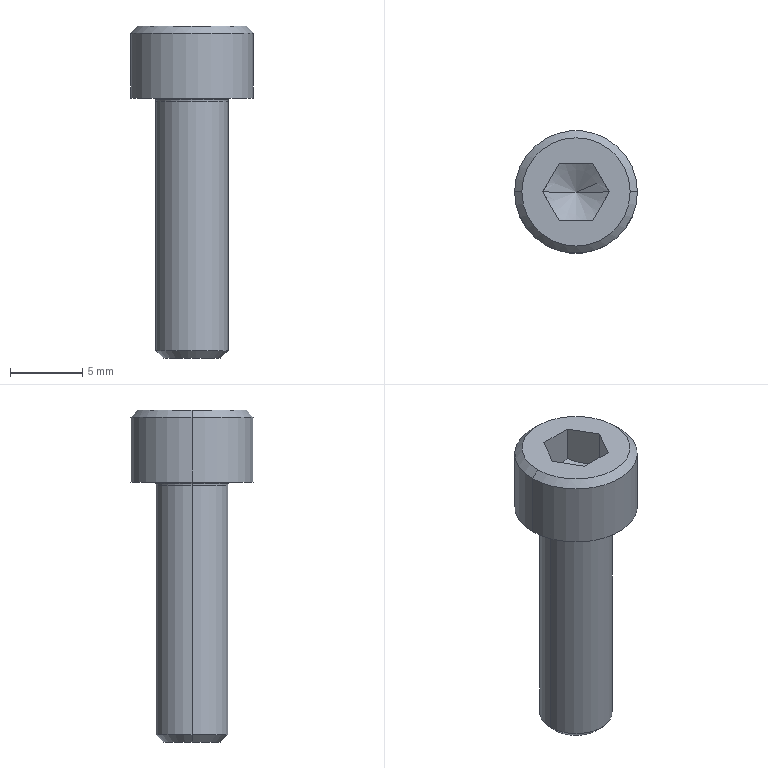Part | Creo | 1 solid | 23 faces | box 8.5 x 8.5 x 23 mm | volume 590.368 mm3 | plane 9 | cone 6 | cylinder 4 | torus 4 | commonest cylinder face diameters 5 x2 8.5 x2
STEP:
#1=CARTESIAN_POINT('',(-237.059,-351.009,-14.5));
#2=VERTEX_POINT('',#1);
#3=CARTESIAN_POINT('',(-238.214,-349.009,-14.5));
#4=VERTEX_POINT('',#3);
#5=CARTESIAN_POINT('',(-237.059,-351.009,-14.5));
#6=CARTESIAN_POINT('',(-237.113,-350.916,-14.531));
#7=CARTESIAN_POINT('',(-237.221,-350.729,-14.587));
#8=CARTESIAN_POINT('',(-237.386,-350.443,-14.648));
#9=CARTESIAN_POINT('',(-237.553,-350.153,-14.68));
#10=CARTESIAN_POINT('',(-237.72,-349.864,-14.68));
#11=CARTESIAN_POINT('',(-237.887,-349.575,-14.648));
#12=CARTESIAN_POINT('',(-238.053,-349.289,-14.587));
#13=CARTESIAN_POINT('',(-238.16,-349.102,-14.531));
#14=CARTESIAN_POINT('',(-238.214,-349.009,-14.5));
#15=B_SPLINE_CURVE_WITH_KNOTS('',3,(#5,#6,#7,#8,#9,#10,#11,#12,#13,#14),.UNSPECIFIED.,.F.,.F.,(4,1,1,1,1,1,1,4),(0.,0.1429,0.2857,0.4286,0.5714,0.7143,0.8571,1.),.UNSPECIFIED.);
#16=EDGE_CURVE('',#2,#4,#15,.T.);
#17=ORIENTED_EDGE('',*,*,#16,.F.);
#18=CARTESIAN_POINT('',(-239.368,-351.009,-15.833));
#19=VERTEX_POINT('',#18);
#20=CARTESIAN_POINT('',(-239.368,-351.009,-15.833));
#21=DIRECTION('',(0.866,0.,0.5));
#22=VECTOR('',#21,2.667);
#23=LINE('',#20,#22);
#24=EDGE_CURVE('',#19,#2,#23,.T.);
#25=ORIENTED_EDGE('',*,*,#24,.F.);
#26=CARTESIAN_POINT('',(-241.678,-351.009,-14.5));
#27=VERTEX_POINT('',#26);
#28=CARTESIAN_POINT('',(-239.368,-351.009,-15.833));
#29=DIRECTION('',(-0.866,0.,0.5));
#30=VECTOR('',#29,2.667);
#31=LINE('',#28,#30);
#32=EDGE_CURVE('',#19,#27,#31,.T.);
#33=ORIENTED_EDGE('',*,*,#32,.T.);
#34=CARTESIAN_POINT('',(-240.523,-349.009,-14.5));
#35=VERTEX_POINT('',#34);
#36=CARTESIAN_POINT('',(-240.523,-349.009,-14.5));
#37=CARTESIAN_POINT('',(-240.577,-349.102,-14.531));
#38=CARTESIAN_POINT('',(-240.685,-349.29,-14.587));
#39=CARTESIAN_POINT('',(-240.85,-349.576,-14.648));
#40=CARTESIAN_POINT('',(-241.017,-349.865,-14.68));
#41=CARTESIAN_POINT('',(-241.185,-350.155,-14.68));
#42=CARTESIAN_POINT('',(-241.351,-350.444,-14.648));
#43=CARTESIAN_POINT('',(-241.517,-350.73,-14.587));
#44=CARTESIAN_POINT('',(-241.624,-350.917,-14.531));
#45=CARTESIAN_POINT('',(-241.678,-351.009,-14.5));
#46=B_SPLINE_CURVE_WITH_KNOTS('',3,(#36,#37,#38,#39,#40,#41,#42,#43,#44,#45),.UNSPECIFIED.,.F.,.F.,(4,1,1,1,1,1,1,4),(0.,0.1429,0.2857,0.4286,0.5714,0.7143,0.8571,1.),.UNSPECIFIED.);
#47=EDGE_CURVE('',#35,#27,#46,.T.);
#48=ORIENTED_EDGE('',*,*,#47,.F.);
#49=CARTESIAN_POINT('',(-238.214,-349.009,-14.5));
#50=CARTESIAN_POINT('',(-238.276,-349.009,-14.518));
#51=CARTESIAN_POINT('',(-238.399,-349.009,-14.551));
#52=CARTESIAN_POINT('',(-238.576,-349.009,-14.592));
#53=CARTESIAN_POINT('',(-238.75,-349.009,-14.626));
#54=CARTESIAN_POINT('',(-238.924,-349.009,-14.652));
#55=CARTESIAN_POINT('',(-239.1,-349.009,-14.67));
#56=CARTESIAN_POINT('',(-239.279,-349.009,-14.679));
#57=CARTESIAN_POINT('',(-239.458,-349.009,-14.679));
#58=CARTESIAN_POINT('',(-239.636,-349.009,-14.67));
#59=CARTESIAN_POINT('',(-239.813,-349.009,-14.652));
#60=CARTESIAN_POINT('',(-239.987,-349.009,-14.626));
#61=CARTESIAN_POINT('',(-240.161,-349.009,-14.592));
#62=CARTESIAN_POINT('',(-240.338,-349.009,-14.551));
#63=CARTESIAN_POINT('',(-240.461,-349.009,-14.518));
#64=CARTESIAN_POINT('',(-240.523,-349.009,-14.5));
#65=B_SPLINE_CURVE_WITH_KNOTS('',3,(#49,#50,#51,#52,#53,#54,#55,#56,#57,#58,#59,#60,#61,#62,#63,#64),.UNSPECIFIED.,.F.,.F.,(4,1,1,1,1,1,1,1,1,1,1,1,1,4),(0.,0.07692,0.1538,0.2308,0.3077,0.3846,0.4615,0.5385,0.6154,0.6923,0.7692,0.8462,0.9231,1.),.UNSPECIFIED.);
#66=EDGE_CURVE('',#4,#35,#65,.T.);
#67=ORIENTED_EDGE('',*,*,#66,.F.);
#68=EDGE_LOOP('',(#17,#25,#33,#48,#67));
#69=FACE_OUTER_BOUND('',#68,.F.);
#70=CARTESIAN_POINT('',(-239.368,-351.009,-15.153));
#71=DIRECTION('',(0.,0.,1.));
#72=DIRECTION('',(1.,0.,0.));
#73=AXIS2_PLACEMENT_3D('',#70,#71,#72);
#74=CONICAL_SURFACE('',#73,1.178,60.);
#75=ADVANCED_FACE('',(#69),#74,.F.);
#76=CARTESIAN_POINT('',(-238.214,-349.009,-12.));
#77=VERTEX_POINT('',#76);
#78=CARTESIAN_POINT('',(-237.059,-351.009,-12.));
#79=VERTEX_POINT('',#78);
#80=CARTESIAN_POINT('',(-238.214,-349.009,-12.));
#81=DIRECTION('',(0.5,-0.866,0.));
#82=VECTOR('',#81,2.309);
#83=LINE('',#80,#82);
#84=EDGE_CURVE('',#77,#79,#83,.T.);
#85=ORIENTED_EDGE('',*,*,#84,.T.);
#86=CARTESIAN_POINT('',(-237.059,-351.009,-12.));
#87=DIRECTION('',(0.,0.,-1.));
#88=VECTOR('',#87,2.5);
#89=LINE('',#86,#88);
#90=EDGE_CURVE('',#79,#2,#89,.T.);
#91=ORIENTED_EDGE('',*,*,#90,.T.);
#92=ORIENTED_EDGE('',*,*,#16,.T.);
#93=CARTESIAN_POINT('',(-238.214,-349.009,-12.));
#94=DIRECTION('',(0.,0.,-1.));
#95=VECTOR('',#94,2.5);
#96=LINE('',#93,#95);
#97=EDGE_CURVE('',#77,#4,#96,.T.);
#98=ORIENTED_EDGE('',*,*,#97,.F.);
#99=EDGE_LOOP('',(#85,#91,#92,#98));
#100=FACE_OUTER_BOUND('',#99,.F.);
#101=CARTESIAN_POINT('',(-238.214,-349.009,-14.5));
#102=DIRECTION('',(-0.866,-0.5,0.));
#103=DIRECTION('',(0.5,-0.866,0.));
#104=AXIS2_PLACEMENT_3D('',#101,#102,#103);
#105=PLANE('',#104);
#106=ADVANCED_FACE('',(#100),#105,.T.);
#107=CARTESIAN_POINT('',(-235.618,-351.009,-12.));
#108=VERTEX_POINT('',#107);
#109=CARTESIAN_POINT('',(-243.118,-351.009,-12.));
#110=VERTEX_POINT('',#109);
#111=CARTESIAN_POINT('',(-239.368,-351.009,-12.));
#112=DIRECTION('',(0.,0.,1.));
#113=DIRECTION('',(1.,0.,0.));
#114=AXIS2_PLACEMENT_3D('',#111,#112,#113);
#115=CIRCLE('',#114,3.75);
#116=EDGE_CURVE('',#108,#110,#115,.T.);
#117=ORIENTED_EDGE('',*,*,#116,.F.);
#118=CARTESIAN_POINT('',(-239.368,-351.009,-12.));
#119=DIRECTION('',(0.,0.,1.));
#120=DIRECTION('',(-1.,0.,0.));
#121=AXIS2_PLACEMENT_3D('',#118,#119,#120);
#122=CIRCLE('',#121,3.75);
#123=EDGE_CURVE('',#110,#108,#122,.T.);
#124=ORIENTED_EDGE('',*,*,#123,.F.);
#125=EDGE_LOOP('',(#117,#124));
#126=FACE_OUTER_BOUND('',#125,.F.);
#127=CARTESIAN_POINT('',(-238.214,-353.009,-12.));
#128=VERTEX_POINT('',#127);
#129=CARTESIAN_POINT('',(-237.059,-351.009,-12.));
#130=DIRECTION('',(-0.5,-0.866,0.));
#131=VECTOR('',#130,2.309);
#132=LINE('',#129,#131);
#133=EDGE_CURVE('',#79,#128,#132,.T.);
#134=ORIENTED_EDGE('',*,*,#133,.F.);
#135=ORIENTED_EDGE('',*,*,#84,.F.);
#136=CARTESIAN_POINT('',(-240.523,-349.009,-12.));
#137=VERTEX_POINT('',#136);
#138=CARTESIAN_POINT('',(-238.214,-349.009,-12.));
#139=DIRECTION('',(-1.,0.,0.));
#140=VECTOR('',#139,2.309);
#141=LINE('',#138,#140);
#142=EDGE_CURVE('',#77,#137,#141,.T.);
#143=ORIENTED_EDGE('',*,*,#142,.T.);
#144=CARTESIAN_POINT('',(-241.678,-351.009,-12.));
#145=VERTEX_POINT('',#144);
#146=CARTESIAN_POINT('',(-241.678,-351.009,-12.));
#147=DIRECTION('',(0.5,0.866,0.));
#148=VECTOR('',#147,2.309);
#149=LINE('',#146,#148);
#150=EDGE_CURVE('',#145,#137,#149,.T.);
#151=ORIENTED_EDGE('',*,*,#150,.F.);
#152=CARTESIAN_POINT('',(-240.523,-353.009,-12.));
#153=VERTEX_POINT('',#152);
#154=CARTESIAN_POINT('',(-240.523,-353.009,-12.));
#155=DIRECTION('',(-0.5,0.866,0.));
#156=VECTOR('',#155,2.309);
#157=LINE('',#154,#156);
#158=EDGE_CURVE('',#153,#145,#157,.T.);
#159=ORIENTED_EDGE('',*,*,#158,.F.);
#160=CARTESIAN_POINT('',(-240.523,-353.009,-12.));
#161=DIRECTION('',(1.,0.,0.));
#162=VECTOR('',#161,2.309);
#163=LINE('',#160,#162);
#164=EDGE_CURVE('',#153,#128,#163,.T.);
#165=ORIENTED_EDGE('',*,*,#164,.T.);
#166=EDGE_LOOP('',(#134,#135,#143,#151,#159,#165));
#167=FACE_BOUND('',#166,.F.);
#168=CARTESIAN_POINT('',(-239.368,-351.009,-12.));
#169=DIRECTION('',(0.,0.,1.));
#170=DIRECTION('',(1.,0.,0.));
#171=AXIS2_PLACEMENT_3D('',#168,#169,#170);
#172=PLANE('',#171);
#173=ADVANCED_FACE('',(#126,#167),#172,.T.);
#174=CARTESIAN_POINT('',(-235.118,-351.009,-12.5));
#175=VERTEX_POINT('',#174);
#176=CARTESIAN_POINT('',(-243.618,-351.009,-12.5));
#177=VERTEX_POINT('',#176);
#178=CARTESIAN_POINT('',(-239.368,-351.009,-12.5));
#179=DIRECTION('',(0.,0.,1.));
#180=DIRECTION('',(1.,0.,0.));
#181=AXIS2_PLACEMENT_3D('',#178,#179,#180);
#182=CIRCLE('',#181,4.25);
#183=EDGE_CURVE('',#175,#177,#182,.T.);
#184=ORIENTED_EDGE('',*,*,#183,.F.);
#185=CARTESIAN_POINT('',(-235.618,-351.009,-12.));
#186=DIRECTION('',(0.7071,0.,-0.7071));
#187=VECTOR('',#186,0.7071);
#188=LINE('',#185,#187);
#189=EDGE_CURVE('',#108,#175,#188,.T.);
#190=ORIENTED_EDGE('',*,*,#189,.F.);
#191=ORIENTED_EDGE('',*,*,#116,.T.);
#192=CARTESIAN_POINT('',(-243.118,-351.009,-12.));
#193=DIRECTION('',(-0.7071,0.,-0.7071));
#194=VECTOR('',#193,0.7071);
#195=LINE('',#192,#194);
#196=EDGE_CURVE('',#110,#177,#195,.T.);
#197=ORIENTED_EDGE('',*,*,#196,.T.);
#198=EDGE_LOOP('',(#184,#190,#191,#197));
#199=FACE_OUTER_BOUND('',#198,.F.);
#200=CARTESIAN_POINT('',(-239.368,-351.009,-12.25));
#201=DIRECTION('',(0.,0.,-1.));
#202=DIRECTION('',(-1.,0.,0.));
#203=AXIS2_PLACEMENT_3D('',#200,#201,#202);
#204=CONICAL_SURFACE('',#203,4.,45.);
#205=ADVANCED_FACE('',(#199),#204,.T.);
#206=ORIENTED_EDGE('',*,*,#183,.T.);
#207=CARTESIAN_POINT('',(-243.618,-351.009,-17.));
#208=VERTEX_POINT('',#207);
#209=CARTESIAN_POINT('',(-243.618,-351.009,-17.));
#210=DIRECTION('',(0.,0.,1.));
#211=VECTOR('',#210,4.5);
#212=LINE('',#209,#211);
#213=EDGE_CURVE('',#208,#177,#212,.T.);
#214=ORIENTED_EDGE('',*,*,#213,.F.);
#215=CARTESIAN_POINT('',(-235.118,-351.009,-17.));
#216=VERTEX_POINT('',#215);
#217=CARTESIAN_POINT('',(-239.368,-351.009,-17.));
#218=DIRECTION('',(0.,0.,-1.));
#219=DIRECTION('',(-1.,0.,0.));
#220=AXIS2_PLACEMENT_3D('',#217,#218,#219);
#221=CIRCLE('',#220,4.25);
#222=EDGE_CURVE('',#208,#216,#221,.T.);
#223=ORIENTED_EDGE('',*,*,#222,.T.);
#224=CARTESIAN_POINT('',(-235.118,-351.009,-17.));
#225=DIRECTION('',(0.,0.,1.));
#226=VECTOR('',#225,4.5);
#227=LINE('',#224,#226);
#228=EDGE_CURVE('',#216,#175,#227,.T.);
#229=ORIENTED_EDGE('',*,*,#228,.T.);
#230=EDGE_LOOP('',(#206,#214,#223,#229));
#231=FACE_OUTER_BOUND('',#230,.F.);
#232=CARTESIAN_POINT('',(-239.368,-351.009,-17.));
#233=DIRECTION('',(0.,0.,1.));
#234=DIRECTION('',(1.,0.,0.));
#235=AXIS2_PLACEMENT_3D('',#232,#233,#234);
#236=CYLINDRICAL_SURFACE('',#235,4.25);
#237=ADVANCED_FACE('',(#231),#236,.T.);
#238=CARTESIAN_POINT('',(-239.368,-351.009,-12.5));
#239=DIRECTION('',(0.,0.,1.));
#240=DIRECTION('',(-1.,0.,0.));
#241=AXIS2_PLACEMENT_3D('',#238,#239,#240);
#242=CIRCLE('',#241,4.25);
#243=EDGE_CURVE('',#177,#175,#242,.T.);
#244=ORIENTED_EDGE('',*,*,#243,.T.);
#245=ORIENTED_EDGE('',*,*,#228,.F.);
#246=CARTESIAN_POINT('',(-239.368,-351.009,-17.));
#247=DIRECTION('',(0.,0.,-1.));
#248=DIRECTION('',(1.,0.,0.));
#249=AXIS2_PLACEMENT_3D('',#246,#247,#248);
#250=CIRCLE('',#249,4.25);
#251=EDGE_CURVE('',#216,#208,#250,.T.);
#252=ORIENTED_EDGE('',*,*,#251,.T.);
#253=ORIENTED_EDGE('',*,*,#213,.T.);
#254=EDGE_LOOP('',(#244,#245,#252,#253));
#255=FACE_OUTER_BOUND('',#254,.F.);
#256=CARTESIAN_POINT('',(-239.368,-351.009,-17.));
#257=DIRECTION('',(0.,0.,1.));
#258=DIRECTION('',(1.,0.,0.));
#259=AXIS2_PLACEMENT_3D('',#256,#257,#258);
#260=CYLINDRICAL_SURFACE('',#259,4.25);
#261=ADVANCED_FACE('',(#255),#260,.T.);
#262=ORIENTED_EDGE('',*,*,#243,.F.);
#263=ORIENTED_EDGE('',*,*,#196,.F.);
#264=ORIENTED_EDGE('',*,*,#123,.T.);
#265=ORIENTED_EDGE('',*,*,#189,.T.);
#266=EDGE_LOOP('',(#262,#263,#264,#265));
#267=FACE_OUTER_BOUND('',#266,.F.);
#268=CARTESIAN_POINT('',(-239.368,-351.009,-12.25));
#269=DIRECTION('',(0.,0.,-1.));
#270=DIRECTION('',(-1.,0.,0.));
#271=AXIS2_PLACEMENT_3D('',#268,#269,#270);
#272=CONICAL_SURFACE('',#271,4.,45.);
#273=ADVANCED_FACE('',(#267),#272,.T.);
#274=ORIENTED_EDGE('',*,*,#251,.F.);
#275=ORIENTED_EDGE('',*,*,#222,.F.);
#276=EDGE_LOOP('',(#274,#275));
#277=FACE_OUTER_BOUND('',#276,.F.);
#278=CARTESIAN_POINT('',(-236.668,-351.009,-17.));
#279=VERTEX_POINT('',#278);
#280=CARTESIAN_POINT('',(-242.068,-351.009,-17.));
#281=VERTEX_POINT('',#280);
#282=CARTESIAN_POINT('',(-239.368,-351.009,-17.));
#283=DIRECTION('',(0.,0.,1.));
#284=DIRECTION('',(1.,0.,0.));
#285=AXIS2_PLACEMENT_3D('',#282,#283,#284);
#286=CIRCLE('',#285,2.7);
#287=EDGE_CURVE('',#279,#281,#286,.T.);
#288=ORIENTED_EDGE('',*,*,#287,.F.);
#289=CARTESIAN_POINT('',(-239.368,-351.009,-17.));
#290=DIRECTION('',(0.,0.,1.));
#291=DIRECTION('',(-1.,0.,0.));
#292=AXIS2_PLACEMENT_3D('',#289,#290,#291);
#293=CIRCLE('',#292,2.7);
#294=EDGE_CURVE('',#281,#279,#293,.T.);
#295=ORIENTED_EDGE('',*,*,#294,.F.);
#296=EDGE_LOOP('',(#288,#295));
#297=FACE_BOUND('',#296,.F.);
#298=CARTESIAN_POINT('',(-239.368,-351.009,-17.));
#299=DIRECTION('',(0.,0.,1.));
#300=DIRECTION('',(1.,0.,0.));
#301=AXIS2_PLACEMENT_3D('',#298,#299,#300);
#302=PLANE('',#301);
#303=ADVANCED_FACE('',(#277,#297),#302,.F.);
#304=ORIENTED_EDGE('',*,*,#287,.T.);
#305=CARTESIAN_POINT('',(-241.927,-351.009,-17.059));
#306=VERTEX_POINT('',#305);
#307=CARTESIAN_POINT('',(-242.068,-351.009,-17.2));
#308=DIRECTION('',(0.,1.,0.));
#309=DIRECTION('',(0.,0.,1.));
#310=AXIS2_PLACEMENT_3D('',#307,#308,#309);
#311=CIRCLE('',#310,0.2);
#312=EDGE_CURVE('',#281,#306,#311,.T.);
#313=ORIENTED_EDGE('',*,*,#312,.T.);
#314=CARTESIAN_POINT('',(-236.81,-351.009,-17.059));
#315=VERTEX_POINT('',#314);
#316=CARTESIAN_POINT('',(-239.368,-351.009,-17.059));
#317=DIRECTION('',(0.,0.,1.));
#318=DIRECTION('',(1.,0.,0.));
#319=AXIS2_PLACEMENT_3D('',#316,#317,#318);
#320=CIRCLE('',#319,2.559);
#321=EDGE_CURVE('',#315,#306,#320,.T.);
#322=ORIENTED_EDGE('',*,*,#321,.F.);
#323=CARTESIAN_POINT('',(-236.668,-351.009,-17.2));
#324=DIRECTION('',(0.,-1.,0.));
#325=DIRECTION('',(0.,0.,1.));
#326=AXIS2_PLACEMENT_3D('',#323,#324,#325);
#327=CIRCLE('',#326,0.2);
#328=EDGE_CURVE('',#279,#315,#327,.T.);
#329=ORIENTED_EDGE('',*,*,#328,.F.);
#330=EDGE_LOOP('',(#304,#313,#322,#329));
#331=FACE_OUTER_BOUND('',#330,.F.);
#332=CARTESIAN_POINT('',(-239.368,-351.009,-17.2));
#333=DIRECTION('',(0.,0.,1.));
#334=DIRECTION('',(1.,0.,0.));
#335=AXIS2_PLACEMENT_3D('',#332,#333,#334);
#336=TOROIDAL_SURFACE('',#335,2.7,0.2);
#337=ADVANCED_FACE('',(#331),#336,.F.);
#338=ORIENTED_EDGE('',*,*,#294,.T.);
#339=ORIENTED_EDGE('',*,*,#328,.T.);
#340=CARTESIAN_POINT('',(-239.368,-351.009,-17.059));
#341=DIRECTION('',(0.,0.,1.));
#342=DIRECTION('',(-1.,0.,0.));
#343=AXIS2_PLACEMENT_3D('',#340,#341,#342);
#344=CIRCLE('',#343,2.559);
#345=EDGE_CURVE('',#306,#315,#344,.T.);
#346=ORIENTED_EDGE('',*,*,#345,.F.);
#347=ORIENTED_EDGE('',*,*,#312,.F.);
#348=EDGE_LOOP('',(#338,#339,#346,#347));
#349=FACE_OUTER_BOUND('',#348,.F.);
#350=CARTESIAN_POINT('',(-239.368,-351.009,-17.2));
#351=DIRECTION('',(0.,0.,1.));
#352=DIRECTION('',(1.,0.,0.));
#353=AXIS2_PLACEMENT_3D('',#350,#351,#352);
#354=TOROIDAL_SURFACE('',#353,2.7,0.2);
#355=ADVANCED_FACE('',(#349),#354,.F.);
#356=CARTESIAN_POINT('',(-241.868,-351.009,-17.2));
#357=VERTEX_POINT('',#356);
#358=CARTESIAN_POINT('',(-236.868,-351.009,-17.2));
#359=VERTEX_POINT('',#358);
#360=CARTESIAN_POINT('',(-239.368,-351.009,-17.2));
#361=DIRECTION('',(0.,0.,1.));
#362=DIRECTION('',(-1.,0.,0.));
#363=AXIS2_PLACEMENT_3D('',#360,#361,#362);
#364=CIRCLE('',#363,2.5);
#365=EDGE_CURVE('',#357,#359,#364,.T.);
#366=ORIENTED_EDGE('',*,*,#365,.F.);
#367=CARTESIAN_POINT('',(-242.068,-351.009,-17.2));
#368=DIRECTION('',(0.,1.,0.));
#369=DIRECTION('',(0.7071,0.,0.7071));
#370=AXIS2_PLACEMENT_3D('',#367,#368,#369);
#371=CIRCLE('',#370,0.2);
#372=EDGE_CURVE('',#306,#357,#371,.T.);
#373=ORIENTED_EDGE('',*,*,#372,.F.);
#374=ORIENTED_EDGE('',*,*,#345,.T.);
#375=CARTESIAN_POINT('',(-236.668,-351.009,-17.2));
#376=DIRECTION('',(0.,-1.,0.));
#377=DIRECTION('',(-0.7071,0.,0.7071));
#378=AXIS2_PLACEMENT_3D('',#375,#376,#377);
#379=CIRCLE('',#378,0.2);
#380=EDGE_CURVE('',#315,#359,#379,.T.);
#381=ORIENTED_EDGE('',*,*,#380,.T.);
#382=EDGE_LOOP('',(#366,#373,#374,#381));
#383=FACE_OUTER_BOUND('',#382,.F.);
#384=CARTESIAN_POINT('',(-239.368,-351.009,-17.2));
#385=DIRECTION('',(0.,0.,1.));
#386=DIRECTION('',(1.,0.,0.));
#387=AXIS2_PLACEMENT_3D('',#384,#385,#386);
#388=TOROIDAL_SURFACE('',#387,2.7,0.2);
#389=ADVANCED_FACE('',(#383),#388,.F.);
#390=CARTESIAN_POINT('',(-236.868,-351.009,-34.5));
#391=VERTEX_POINT('',#390);
#392=CARTESIAN_POINT('',(-241.868,-351.009,-34.5));
#393=VERTEX_POINT('',#392);
#394=CARTESIAN_POINT('',(-239.368,-351.009,-34.5));
#395=DIRECTION('',(0.,0.,-1.));
#396=DIRECTION('',(1.,0.,0.));
#397=AXIS2_PLACEMENT_3D('',#394,#395,#396);
#398=CIRCLE('',#397,2.5);
#399=EDGE_CURVE('',#391,#393,#398,.T.);
#400=ORIENTED_EDGE('',*,*,#399,.T.);
#401=CARTESIAN_POINT('',(-241.868,-351.009,-34.5));
#402=DIRECTION('',(0.,0.,1.));
#403=VECTOR('',#402,17.3);
#404=LINE('',#401,#403);
#405=EDGE_CURVE('',#393,#357,#404,.T.);
#406=ORIENTED_EDGE('',*,*,#405,.T.);
#407=ORIENTED_EDGE('',*,*,#365,.T.);
#408=CARTESIAN_POINT('',(-236.868,-351.009,-34.5));
#409=DIRECTION('',(0.,0.,1.));
#410=VECTOR('',#409,17.3);
#411=LINE('',#408,#410);
#412=EDGE_CURVE('',#391,#359,#411,.T.);
#413=ORIENTED_EDGE('',*,*,#412,.F.);
#414=EDGE_LOOP('',(#400,#406,#407,#413));
#415=FACE_OUTER_BOUND('',#414,.F.);
#416=CARTESIAN_POINT('',(-239.368,-351.009,-35.));
#417=DIRECTION('',(0.,0.,1.));
#418=DIRECTION('',(1.,0.,0.));
#419=AXIS2_PLACEMENT_3D('',#416,#417,#418);
#420=CYLINDRICAL_SURFACE('',#419,2.5);
#421=ADVANCED_FACE('',(#415),#420,.T.);
#422=CARTESIAN_POINT('',(-237.368,-351.009,-35.));
#423=VERTEX_POINT('',#422);
#424=CARTESIAN_POINT('',(-241.368,-351.009,-35.));
#425=VERTEX_POINT('',#424);
#426=CARTESIAN_POINT('',(-239.368,-351.009,-35.));
#427=DIRECTION('',(0.,0.,-1.));
#428=DIRECTION('',(1.,0.,0.));
#429=AXIS2_PLACEMENT_3D('',#426,#427,#428);
#430=CIRCLE('',#429,2.);
#431=EDGE_CURVE('',#423,#425,#430,.T.);
#432=ORIENTED_EDGE('',*,*,#431,.T.);
#433=CARTESIAN_POINT('',(-241.368,-351.009,-35.));
#434=DIRECTION('',(-0.7071,0.,0.7071));
#435=VECTOR('',#434,0.7071);
#436=LINE('',#433,#435);
#437=EDGE_CURVE('',#425,#393,#436,.T.);
#438=ORIENTED_EDGE('',*,*,#437,.T.);
#439=ORIENTED_EDGE('',*,*,#399,.F.);
#440=CARTESIAN_POINT('',(-237.368,-351.009,-35.));
#441=DIRECTION('',(0.7071,0.,0.7071));
#442=VECTOR('',#441,0.7071);
#443=LINE('',#440,#442);
#444=EDGE_CURVE('',#423,#391,#443,.T.);
#445=ORIENTED_EDGE('',*,*,#444,.F.);
#446=EDGE_LOOP('',(#432,#438,#439,#445));
#447=FACE_OUTER_BOUND('',#446,.F.);
#448=CARTESIAN_POINT('',(-239.368,-351.009,-34.75));
#449=DIRECTION('',(0.,0.,1.));
#450=DIRECTION('',(1.,0.,0.));
#451=AXIS2_PLACEMENT_3D('',#448,#449,#450);
#452=CONICAL_SURFACE('',#451,2.25,45.);
#453=ADVANCED_FACE('',(#447),#452,.T.);
#454=ORIENTED_EDGE('',*,*,#431,.F.);
#455=CARTESIAN_POINT('',(-239.368,-351.009,-35.));
#456=DIRECTION('',(0.,0.,-1.));
#457=DIRECTION('',(-1.,0.,0.));
#458=AXIS2_PLACEMENT_3D('',#455,#456,#457);
#459=CIRCLE('',#458,2.);
#460=EDGE_CURVE('',#425,#423,#459,.T.);
#461=ORIENTED_EDGE('',*,*,#460,.F.);
#462=EDGE_LOOP('',(#454,#461));
#463=FACE_OUTER_BOUND('',#462,.F.);
#464=CARTESIAN_POINT('',(-239.368,-351.009,-35.));
#465=DIRECTION('',(0.,0.,1.));
#466=DIRECTION('',(1.,0.,0.));
#467=AXIS2_PLACEMENT_3D('',#464,#465,#466);
#468=PLANE('',#467);
#469=ADVANCED_FACE('',(#463),#468,.F.);
#470=ORIENTED_EDGE('',*,*,#460,.T.);
#471=ORIENTED_EDGE('',*,*,#444,.T.);
#472=CARTESIAN_POINT('',(-239.368,-351.009,-34.5));
#473=DIRECTION('',(0.,0.,-1.));
#474=DIRECTION('',(-1.,0.,0.));
#475=AXIS2_PLACEMENT_3D('',#472,#473,#474);
#476=CIRCLE('',#475,2.5);
#477=EDGE_CURVE('',#393,#391,#476,.T.);
#478=ORIENTED_EDGE('',*,*,#477,.F.);
#479=ORIENTED_EDGE('',*,*,#437,.F.);
#480=EDGE_LOOP('',(#470,#471,#478,#479));
#481=FACE_OUTER_BOUND('',#480,.F.);
#482=CARTESIAN_POINT('',(-239.368,-351.009,-34.75));
#483=DIRECTION('',(0.,0.,1.));
#484=DIRECTION('',(1.,0.,0.));
#485=AXIS2_PLACEMENT_3D('',#482,#483,#484);
#486=CONICAL_SURFACE('',#485,2.25,45.);
#487=ADVANCED_FACE('',(#481),#486,.T.);
#488=ORIENTED_EDGE('',*,*,#477,.T.);
#489=ORIENTED_EDGE('',*,*,#412,.T.);
#490=CARTESIAN_POINT('',(-239.368,-351.009,-17.2));
#491=DIRECTION('',(0.,0.,1.));
#492=DIRECTION('',(1.,0.,0.));
#493=AXIS2_PLACEMENT_3D('',#490,#491,#492);
#494=CIRCLE('',#493,2.5);
#495=EDGE_CURVE('',#359,#357,#494,.T.);
#496=ORIENTED_EDGE('',*,*,#495,.T.);
#497=ORIENTED_EDGE('',*,*,#405,.F.);
#498=EDGE_LOOP('',(#488,#489,#496,#497));
#499=FACE_OUTER_BOUND('',#498,.F.);
#500=CARTESIAN_POINT('',(-239.368,-351.009,-35.));
#501=DIRECTION('',(0.,0.,1.));
#502=DIRECTION('',(1.,0.,0.));
#503=AXIS2_PLACEMENT_3D('',#500,#501,#502);
#504=CYLINDRICAL_SURFACE('',#503,2.5);
#505=ADVANCED_FACE('',(#499),#504,.T.);
#506=ORIENTED_EDGE('',*,*,#495,.F.);
#507=ORIENTED_EDGE('',*,*,#380,.F.);
#508=ORIENTED_EDGE('',*,*,#321,.T.);
#509=ORIENTED_EDGE('',*,*,#372,.T.);
#510=EDGE_LOOP('',(#506,#507,#508,#509));
#511=FACE_OUTER_BOUND('',#510,.F.);
#512=CARTESIAN_POINT('',(-239.368,-351.009,-17.2));
#513=DIRECTION('',(0.,0.,1.));
#514=DIRECTION('',(1.,0.,0.));
#515=AXIS2_PLACEMENT_3D('',#512,#513,#514);
#516=TOROIDAL_SURFACE('',#515,2.7,0.2);
#517=ADVANCED_FACE('',(#511),#516,.F.);
#518=ORIENTED_EDGE('',*,*,#133,.T.);
#519=CARTESIAN_POINT('',(-238.214,-353.009,-14.5));
#520=VERTEX_POINT('',#519);
#521=CARTESIAN_POINT('',(-238.214,-353.009,-12.));
#522=DIRECTION('',(0.,0.,-1.));
#523=VECTOR('',#522,2.5);
#524=LINE('',#521,#523);
#525=EDGE_CURVE('',#128,#520,#524,.T.);
#526=ORIENTED_EDGE('',*,*,#525,.T.);
#527=CARTESIAN_POINT('',(-238.214,-353.009,-14.5));
#528=CARTESIAN_POINT('',(-238.16,-352.916,-14.531));
#529=CARTESIAN_POINT('',(-238.052,-352.729,-14.587));
#530=CARTESIAN_POINT('',(-237.887,-352.443,-14.648));
#531=CARTESIAN_POINT('',(-237.72,-352.153,-14.68));
#532=CARTESIAN_POINT('',(-237.552,-351.864,-14.68));
#533=CARTESIAN_POINT('',(-237.385,-351.575,-14.648));
#534=CARTESIAN_POINT('',(-237.22,-351.289,-14.587));
#535=CARTESIAN_POINT('',(-237.113,-351.102,-14.531));
#536=CARTESIAN_POINT('',(-237.059,-351.009,-14.5));
#537=B_SPLINE_CURVE_WITH_KNOTS('',3,(#527,#528,#529,#530,#531,#532,#533,#534,#535,#536),.UNSPECIFIED.,.F.,.F.,(4,1,1,1,1,1,1,4),(0.,0.1429,0.2857,0.4286,0.5714,0.7143,0.8571,1.),.UNSPECIFIED.);
#538=EDGE_CURVE('',#520,#2,#537,.T.);
#539=ORIENTED_EDGE('',*,*,#538,.T.);
#540=ORIENTED_EDGE('',*,*,#90,.F.);
#541=EDGE_LOOP('',(#518,#526,#539,#540));
#542=FACE_OUTER_BOUND('',#541,.F.);
#543=CARTESIAN_POINT('',(-237.059,-351.009,-14.5));
#544=DIRECTION('',(-0.866,0.5,0.));
#545=DIRECTION('',(-0.5,-0.866,0.));
#546=AXIS2_PLACEMENT_3D('',#543,#544,#545);
#547=PLANE('',#546);
#548=ADVANCED_FACE('',(#542),#547,.T.);
#549=ORIENTED_EDGE('',*,*,#164,.F.);
#550=CARTESIAN_POINT('',(-240.523,-353.009,-14.5));
#551=VERTEX_POINT('',#550);
#552=CARTESIAN_POINT('',(-240.523,-353.009,-12.));
#553=DIRECTION('',(0.,0.,-1.));
#554=VECTOR('',#553,2.5);
#555=LINE('',#552,#554);
#556=EDGE_CURVE('',#153,#551,#555,.T.);
#557=ORIENTED_EDGE('',*,*,#556,.T.);
#558=CARTESIAN_POINT('',(-240.523,-353.009,-14.5));
#559=CARTESIAN_POINT('',(-240.461,-353.009,-14.518));
#560=CARTESIAN_POINT('',(-240.338,-353.009,-14.551));
#561=CARTESIAN_POINT('',(-240.161,-353.009,-14.592));
#562=CARTESIAN_POINT('',(-239.987,-353.009,-14.626));
#563=CARTESIAN_POINT('',(-239.813,-353.009,-14.652));
#564=CARTESIAN_POINT('',(-239.636,-353.009,-14.67));
#565=CARTESIAN_POINT('',(-239.458,-353.009,-14.679));
#566=CARTESIAN_POINT('',(-239.279,-353.009,-14.679));
#567=CARTESIAN_POINT('',(-239.1,-353.009,-14.67));
#568=CARTESIAN_POINT('',(-238.924,-353.009,-14.652));
#569=CARTESIAN_POINT('',(-238.75,-353.009,-14.626));
#570=CARTESIAN_POINT('',(-238.576,-353.009,-14.592));
#571=CARTESIAN_POINT('',(-238.399,-353.009,-14.551));
#572=CARTESIAN_POINT('',(-238.276,-353.009,-14.518));
#573=CARTESIAN_POINT('',(-238.214,-353.009,-14.5));
#574=B_SPLINE_CURVE_WITH_KNOTS('',3,(#558,#559,#560,#561,#562,#563,#564,#565,#566,#567,#568,#569,#570,#571,#572,#573),.UNSPECIFIED.,.F.,.F.,(4,1,1,1,1,1,1,1,1,1,1,1,1,4),(0.,0.07692,0.1538,0.2308,0.3077,0.3846,0.4615,0.5385,0.6154,0.6923,0.7692,0.8462,0.9231,1.),.UNSPECIFIED.);
#575=EDGE_CURVE('',#551,#520,#574,.T.);
#576=ORIENTED_EDGE('',*,*,#575,.T.);
#577=ORIENTED_EDGE('',*,*,#525,.F.);
#578=EDGE_LOOP('',(#549,#557,#576,#577));
#579=FACE_OUTER_BOUND('',#578,.F.);
#580=CARTESIAN_POINT('',(-238.214,-353.009,-14.5));
#581=DIRECTION('',(0.,1.,0.));
#582=DIRECTION('',(0.,0.,1.));
#583=AXIS2_PLACEMENT_3D('',#580,#581,#582);
#584=PLANE('',#583);
#585=ADVANCED_FACE('',(#579),#584,.T.);
#586=ORIENTED_EDGE('',*,*,#158,.T.);
#587=CARTESIAN_POINT('',(-241.678,-351.009,-12.));
#588=DIRECTION('',(0.,0.,-1.));
#589=VECTOR('',#588,2.5);
#590=LINE('',#587,#589);
#591=EDGE_CURVE('',#145,#27,#590,.T.);
#592=ORIENTED_EDGE('',*,*,#591,.T.);
#593=CARTESIAN_POINT('',(-241.678,-351.009,-14.5));
#594=CARTESIAN_POINT('',(-241.624,-351.102,-14.531));
#595=CARTESIAN_POINT('',(-241.517,-351.289,-14.587));
#596=CARTESIAN_POINT('',(-241.351,-351.575,-14.648));
#597=CARTESIAN_POINT('',(-241.185,-351.864,-14.68));
#598=CARTESIAN_POINT('',(-241.017,-352.153,-14.68));
#599=CARTESIAN_POINT('',(-240.85,-352.443,-14.648));
#600=CARTESIAN_POINT('',(-240.685,-352.729,-14.587));
#601=CARTESIAN_POINT('',(-240.577,-352.916,-14.531));
#602=CARTESIAN_POINT('',(-240.523,-353.009,-14.5));
#603=B_SPLINE_CURVE_WITH_KNOTS('',3,(#593,#594,#595,#596,#597,#598,#599,#600,#601,#602),.UNSPECIFIED.,.F.,.F.,(4,1,1,1,1,1,1,4),(0.,0.1429,0.2857,0.4286,0.5714,0.7143,0.8571,1.),.UNSPECIFIED.);
#604=EDGE_CURVE('',#27,#551,#603,.T.);
#605=ORIENTED_EDGE('',*,*,#604,.T.);
#606=ORIENTED_EDGE('',*,*,#556,.F.);
#607=EDGE_LOOP('',(#586,#592,#605,#606));
#608=FACE_OUTER_BOUND('',#607,.F.);
#609=CARTESIAN_POINT('',(-240.523,-353.009,-14.5));
#610=DIRECTION('',(0.866,0.5,0.));
#611=DIRECTION('',(-0.5,0.866,0.));
#612=AXIS2_PLACEMENT_3D('',#609,#610,#611);
#613=PLANE('',#612);
#614=ADVANCED_FACE('',(#608),#613,.T.);
#615=ORIENTED_EDGE('',*,*,#150,.T.);
#616=CARTESIAN_POINT('',(-240.523,-349.009,-12.));
#617=DIRECTION('',(0.,0.,-1.));
#618=VECTOR('',#617,2.5);
#619=LINE('',#616,#618);
#620=EDGE_CURVE('',#137,#35,#619,.T.);
#621=ORIENTED_EDGE('',*,*,#620,.T.);
#622=ORIENTED_EDGE('',*,*,#47,.T.);
#623=ORIENTED_EDGE('',*,*,#591,.F.);
#624=EDGE_LOOP('',(#615,#621,#622,#623));
#625=FACE_OUTER_BOUND('',#624,.F.);
#626=CARTESIAN_POINT('',(-241.678,-351.009,-14.5));
#627=DIRECTION('',(0.866,-0.5,0.));
#628=DIRECTION('',(0.5,0.866,0.));
#629=AXIS2_PLACEMENT_3D('',#626,#627,#628);
#630=PLANE('',#629);
#631=ADVANCED_FACE('',(#625),#630,.T.);
#632=ORIENTED_EDGE('',*,*,#142,.F.);
#633=ORIENTED_EDGE('',*,*,#97,.T.);
#634=ORIENTED_EDGE('',*,*,#66,.T.);
#635=ORIENTED_EDGE('',*,*,#620,.F.);
#636=EDGE_LOOP('',(#632,#633,#634,#635));
#637=FACE_OUTER_BOUND('',#636,.F.);
#638=CARTESIAN_POINT('',(-240.523,-349.009,-14.5));
#639=DIRECTION('',(0.,-1.,0.));
#640=DIRECTION('',(0.,0.,-1.));
#641=AXIS2_PLACEMENT_3D('',#638,#639,#640);
#642=PLANE('',#641);
#643=ADVANCED_FACE('',(#637),#642,.T.);
#644=ORIENTED_EDGE('',*,*,#604,.F.);
#645=ORIENTED_EDGE('',*,*,#32,.F.);
#646=ORIENTED_EDGE('',*,*,#24,.T.);
#647=ORIENTED_EDGE('',*,*,#538,.F.);
#648=ORIENTED_EDGE('',*,*,#575,.F.);
#649=EDGE_LOOP('',(#644,#645,#646,#647,#648));
#650=FACE_OUTER_BOUND('',#649,.F.);
#651=CARTESIAN_POINT('',(-239.368,-351.009,-15.153));
#652=DIRECTION('',(0.,0.,1.));
#653=DIRECTION('',(1.,0.,0.));
#654=AXIS2_PLACEMENT_3D('',#651,#652,#653);
#655=CONICAL_SURFACE('',#654,1.178,60.);
#656=ADVANCED_FACE('',(#650),#655,.F.);
#657=CLOSED_SHELL('',(#75,#106,#173,#205,#237,#261,#273,#303,#337,#355,#389,#421,#453,#469,#487,#505,#517,#548,#585,#614,#631,#643,#656));
#658=MANIFOLD_SOLID_BREP('',#657);
#659=(LENGTH_UNIT()NAMED_UNIT(*)SI_UNIT(.MILLI.,.METRE.));
#660=UNCERTAINTY_MEASURE_WITH_UNIT(LENGTH_MEASURE(0.002595),#659,'','');
#661=(NAMED_UNIT(*)PLANE_ANGLE_UNIT()SI_UNIT($,.RADIAN.));
#662=PLANE_ANGLE_MEASURE_WITH_UNIT(PLANE_ANGLE_MEASURE(0.01745),#661);
#663=(CONVERSION_BASED_UNIT('DEGREE',#662)NAMED_UNIT(*)PLANE_ANGLE_UNIT());
#664=(NAMED_UNIT(*)SI_UNIT($,.STERADIAN.)SOLID_ANGLE_UNIT());
#665=(GEOMETRIC_REPRESENTATION_CONTEXT(3)GLOBAL_UNCERTAINTY_ASSIGNED_CONTEXT((#660))GLOBAL_UNIT_ASSIGNED_CONTEXT((#659,#663,#664))REPRESENTATION_CONTEXT('',''));
#666=ADVANCED_BREP_SHAPE_REPRESENTATION('',(#658),#665);